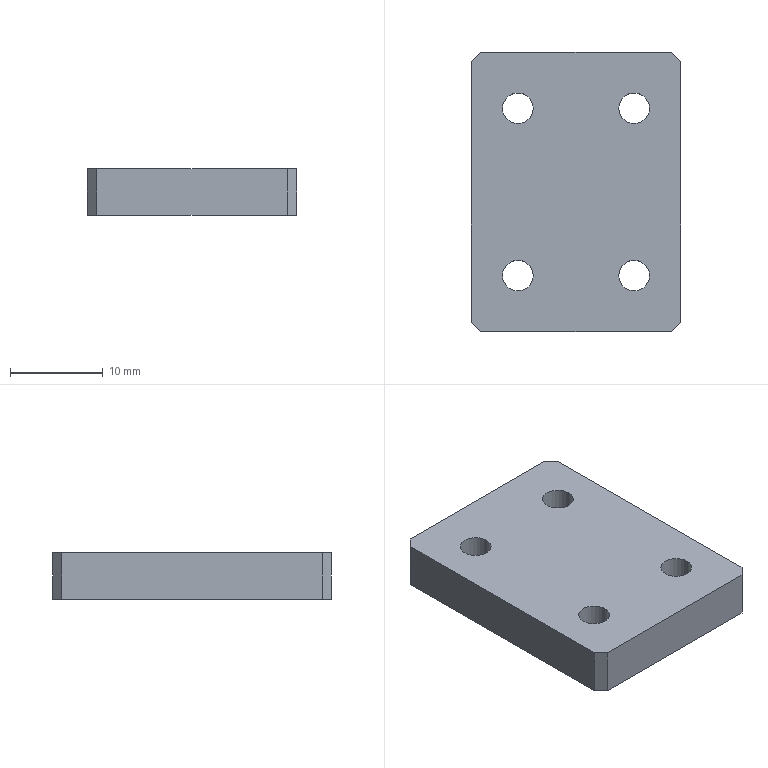Part | STEP file | 01-07 loading cylinder pad plate | 1 solid | 18 faces | box 22.5 x 30 x 5 mm | volume 3194 mm3 | plane 10 | cylinder 8 | commonest cylinder face diameters 3.3 x8
STEP:
#1=CARTESIAN_POINT('',(4.6,-9.,5.));
#2=VERTEX_POINT('',#1);
#3=CARTESIAN_POINT('',(7.9,-9.,5.));
#4=VERTEX_POINT('',#3);
#5=CARTESIAN_POINT('',(6.25,-9.,5.));
#6=DIRECTION('',(0.,0.,1.));
#7=DIRECTION('',(1.,0.,0.));
#8=AXIS2_PLACEMENT_3D('',#5,#6,#7);
#9=CIRCLE('',#8,1.65);
#10=EDGE_CURVE('',#2,#4,#9,.T.);
#11=ORIENTED_EDGE('',*,*,#10,.T.);
#12=CARTESIAN_POINT('',(7.9,-9.,0.));
#13=VERTEX_POINT('',#12);
#14=CARTESIAN_POINT('',(7.9,-9.,0.));
#15=DIRECTION('',(0.,0.,-1.));
#16=VECTOR('',#15,1000.);
#17=LINE('',#14,#16);
#18=EDGE_CURVE('',#4,#13,#17,.T.);
#19=ORIENTED_EDGE('',*,*,#18,.T.);
#20=CARTESIAN_POINT('',(4.6,-9.,0.));
#21=VERTEX_POINT('',#20);
#22=CARTESIAN_POINT('',(6.25,-9.,0.));
#23=DIRECTION('',(0.,0.,-1.));
#24=DIRECTION('',(-1.,0.,0.));
#25=AXIS2_PLACEMENT_3D('',#22,#23,#24);
#26=CIRCLE('',#25,1.65);
#27=EDGE_CURVE('',#13,#21,#26,.T.);
#28=ORIENTED_EDGE('',*,*,#27,.T.);
#29=CARTESIAN_POINT('',(4.6,-9.,0.));
#30=DIRECTION('',(0.,0.,-1.));
#31=VECTOR('',#30,1000.);
#32=LINE('',#29,#31);
#33=EDGE_CURVE('',#2,#21,#32,.T.);
#34=ORIENTED_EDGE('',*,*,#33,.F.);
#35=EDGE_LOOP('',(#11,#19,#28,#34));
#36=FACE_OUTER_BOUND('',#35,.T.);
#37=CARTESIAN_POINT('',(6.25,-9.,0.));
#38=DIRECTION('',(0.,0.,-1.));
#39=DIRECTION('',(-1.,0.,0.));
#40=AXIS2_PLACEMENT_3D('',#37,#38,#39);
#41=CYLINDRICAL_SURFACE('',#40,1.65);
#42=ADVANCED_FACE('',(#36),#41,.F.);
#43=CARTESIAN_POINT('',(-7.9,-9.,5.));
#44=VERTEX_POINT('',#43);
#45=CARTESIAN_POINT('',(-4.6,-9.,5.));
#46=VERTEX_POINT('',#45);
#47=CARTESIAN_POINT('',(-6.25,-9.,5.));
#48=DIRECTION('',(0.,0.,1.));
#49=DIRECTION('',(1.,0.,0.));
#50=AXIS2_PLACEMENT_3D('',#47,#48,#49);
#51=CIRCLE('',#50,1.65);
#52=EDGE_CURVE('',#44,#46,#51,.T.);
#53=ORIENTED_EDGE('',*,*,#52,.T.);
#54=CARTESIAN_POINT('',(-4.6,-9.,0.));
#55=VERTEX_POINT('',#54);
#56=CARTESIAN_POINT('',(-4.6,-9.,0.));
#57=DIRECTION('',(0.,0.,-1.));
#58=VECTOR('',#57,1000.);
#59=LINE('',#56,#58);
#60=EDGE_CURVE('',#46,#55,#59,.T.);
#61=ORIENTED_EDGE('',*,*,#60,.T.);
#62=CARTESIAN_POINT('',(-7.9,-9.,0.));
#63=VERTEX_POINT('',#62);
#64=CARTESIAN_POINT('',(-6.25,-9.,0.));
#65=DIRECTION('',(0.,0.,-1.));
#66=DIRECTION('',(-1.,0.,0.));
#67=AXIS2_PLACEMENT_3D('',#64,#65,#66);
#68=CIRCLE('',#67,1.65);
#69=EDGE_CURVE('',#55,#63,#68,.T.);
#70=ORIENTED_EDGE('',*,*,#69,.T.);
#71=CARTESIAN_POINT('',(-7.9,-9.,0.));
#72=DIRECTION('',(0.,0.,-1.));
#73=VECTOR('',#72,1000.);
#74=LINE('',#71,#73);
#75=EDGE_CURVE('',#44,#63,#74,.T.);
#76=ORIENTED_EDGE('',*,*,#75,.F.);
#77=EDGE_LOOP('',(#53,#61,#70,#76));
#78=FACE_OUTER_BOUND('',#77,.T.);
#79=CARTESIAN_POINT('',(-6.25,-9.,0.));
#80=DIRECTION('',(0.,0.,-1.));
#81=DIRECTION('',(-1.,0.,0.));
#82=AXIS2_PLACEMENT_3D('',#79,#80,#81);
#83=CYLINDRICAL_SURFACE('',#82,1.65);
#84=ADVANCED_FACE('',(#78),#83,.F.);
#85=CARTESIAN_POINT('',(-7.9,9.,5.));
#86=VERTEX_POINT('',#85);
#87=CARTESIAN_POINT('',(-4.6,9.,5.));
#88=VERTEX_POINT('',#87);
#89=CARTESIAN_POINT('',(-6.25,9.,5.));
#90=DIRECTION('',(0.,0.,1.));
#91=DIRECTION('',(1.,0.,0.));
#92=AXIS2_PLACEMENT_3D('',#89,#90,#91);
#93=CIRCLE('',#92,1.65);
#94=EDGE_CURVE('',#86,#88,#93,.T.);
#95=ORIENTED_EDGE('',*,*,#94,.T.);
#96=CARTESIAN_POINT('',(-4.6,9.,0.));
#97=VERTEX_POINT('',#96);
#98=CARTESIAN_POINT('',(-4.6,9.,0.));
#99=DIRECTION('',(0.,0.,-1.));
#100=VECTOR('',#99,1000.);
#101=LINE('',#98,#100);
#102=EDGE_CURVE('',#88,#97,#101,.T.);
#103=ORIENTED_EDGE('',*,*,#102,.T.);
#104=CARTESIAN_POINT('',(-7.9,9.,0.));
#105=VERTEX_POINT('',#104);
#106=CARTESIAN_POINT('',(-6.25,9.,0.));
#107=DIRECTION('',(0.,0.,-1.));
#108=DIRECTION('',(-1.,0.,0.));
#109=AXIS2_PLACEMENT_3D('',#106,#107,#108);
#110=CIRCLE('',#109,1.65);
#111=EDGE_CURVE('',#97,#105,#110,.T.);
#112=ORIENTED_EDGE('',*,*,#111,.T.);
#113=CARTESIAN_POINT('',(-7.9,9.,0.));
#114=DIRECTION('',(0.,0.,-1.));
#115=VECTOR('',#114,1000.);
#116=LINE('',#113,#115);
#117=EDGE_CURVE('',#86,#105,#116,.T.);
#118=ORIENTED_EDGE('',*,*,#117,.F.);
#119=EDGE_LOOP('',(#95,#103,#112,#118));
#120=FACE_OUTER_BOUND('',#119,.T.);
#121=CARTESIAN_POINT('',(-6.25,9.,0.));
#122=DIRECTION('',(0.,0.,-1.));
#123=DIRECTION('',(-1.,0.,0.));
#124=AXIS2_PLACEMENT_3D('',#121,#122,#123);
#125=CYLINDRICAL_SURFACE('',#124,1.65);
#126=ADVANCED_FACE('',(#120),#125,.F.);
#127=CARTESIAN_POINT('',(4.6,9.,5.));
#128=VERTEX_POINT('',#127);
#129=CARTESIAN_POINT('',(7.9,9.,5.));
#130=VERTEX_POINT('',#129);
#131=CARTESIAN_POINT('',(6.25,9.,5.));
#132=DIRECTION('',(0.,0.,1.));
#133=DIRECTION('',(1.,0.,0.));
#134=AXIS2_PLACEMENT_3D('',#131,#132,#133);
#135=CIRCLE('',#134,1.65);
#136=EDGE_CURVE('',#128,#130,#135,.T.);
#137=ORIENTED_EDGE('',*,*,#136,.T.);
#138=CARTESIAN_POINT('',(7.9,9.,0.));
#139=VERTEX_POINT('',#138);
#140=CARTESIAN_POINT('',(7.9,9.,0.));
#141=DIRECTION('',(0.,0.,-1.));
#142=VECTOR('',#141,1000.);
#143=LINE('',#140,#142);
#144=EDGE_CURVE('',#130,#139,#143,.T.);
#145=ORIENTED_EDGE('',*,*,#144,.T.);
#146=CARTESIAN_POINT('',(4.6,9.,0.));
#147=VERTEX_POINT('',#146);
#148=CARTESIAN_POINT('',(6.25,9.,0.));
#149=DIRECTION('',(0.,0.,-1.));
#150=DIRECTION('',(-1.,0.,0.));
#151=AXIS2_PLACEMENT_3D('',#148,#149,#150);
#152=CIRCLE('',#151,1.65);
#153=EDGE_CURVE('',#139,#147,#152,.T.);
#154=ORIENTED_EDGE('',*,*,#153,.T.);
#155=CARTESIAN_POINT('',(4.6,9.,0.));
#156=DIRECTION('',(0.,0.,-1.));
#157=VECTOR('',#156,1000.);
#158=LINE('',#155,#157);
#159=EDGE_CURVE('',#128,#147,#158,.T.);
#160=ORIENTED_EDGE('',*,*,#159,.F.);
#161=EDGE_LOOP('',(#137,#145,#154,#160));
#162=FACE_OUTER_BOUND('',#161,.T.);
#163=CARTESIAN_POINT('',(6.25,9.,0.));
#164=DIRECTION('',(0.,0.,-1.));
#165=DIRECTION('',(-1.,0.,0.));
#166=AXIS2_PLACEMENT_3D('',#163,#164,#165);
#167=CYLINDRICAL_SURFACE('',#166,1.65);
#168=ADVANCED_FACE('',(#162),#167,.F.);
#169=CARTESIAN_POINT('',(11.25,-14.,5.));
#170=VERTEX_POINT('',#169);
#171=CARTESIAN_POINT('',(11.25,14.,5.));
#172=VERTEX_POINT('',#171);
#173=CARTESIAN_POINT('',(11.25,15.,5.));
#174=DIRECTION('',(0.,1.,0.));
#175=VECTOR('',#174,1000.);
#176=LINE('',#173,#175);
#177=EDGE_CURVE('',#170,#172,#176,.T.);
#178=ORIENTED_EDGE('',*,*,#177,.F.);
#179=CARTESIAN_POINT('',(11.25,-14.,0.));
#180=VERTEX_POINT('',#179);
#181=CARTESIAN_POINT('',(11.25,-14.,5.));
#182=DIRECTION('',(0.,0.,-1.));
#183=VECTOR('',#182,1000.);
#184=LINE('',#181,#183);
#185=EDGE_CURVE('',#170,#180,#184,.T.);
#186=ORIENTED_EDGE('',*,*,#185,.T.);
#187=CARTESIAN_POINT('',(11.25,14.,0.));
#188=VERTEX_POINT('',#187);
#189=CARTESIAN_POINT('',(11.25,15.,0.));
#190=DIRECTION('',(0.,1.,0.));
#191=VECTOR('',#190,1000.);
#192=LINE('',#189,#191);
#193=EDGE_CURVE('',#180,#188,#192,.T.);
#194=ORIENTED_EDGE('',*,*,#193,.T.);
#195=CARTESIAN_POINT('',(11.25,14.,5.));
#196=DIRECTION('',(0.,0.,1.));
#197=VECTOR('',#196,1000.);
#198=LINE('',#195,#197);
#199=EDGE_CURVE('',#188,#172,#198,.T.);
#200=ORIENTED_EDGE('',*,*,#199,.T.);
#201=EDGE_LOOP('',(#178,#186,#194,#200));
#202=FACE_OUTER_BOUND('',#201,.T.);
#203=CARTESIAN_POINT('',(11.25,15.,5.));
#204=DIRECTION('',(-1.,0.,0.));
#205=DIRECTION('',(0.,-1.,0.));
#206=AXIS2_PLACEMENT_3D('',#203,#204,#205);
#207=PLANE('',#206);
#208=ADVANCED_FACE('',(#202),#207,.F.);
#209=CARTESIAN_POINT('',(10.25,15.,0.));
#210=VERTEX_POINT('',#209);
#211=CARTESIAN_POINT('',(-10.25,15.,0.));
#212=VERTEX_POINT('',#211);
#213=CARTESIAN_POINT('',(-11.25,15.,0.));
#214=DIRECTION('',(-1.,0.,0.));
#215=VECTOR('',#214,1000.);
#216=LINE('',#213,#215);
#217=EDGE_CURVE('',#210,#212,#216,.T.);
#218=ORIENTED_EDGE('',*,*,#217,.T.);
#219=CARTESIAN_POINT('',(-10.25,15.,5.));
#220=VERTEX_POINT('',#219);
#221=CARTESIAN_POINT('',(-10.25,15.,5.));
#222=DIRECTION('',(0.,0.,1.));
#223=VECTOR('',#222,1000.);
#224=LINE('',#221,#223);
#225=EDGE_CURVE('',#212,#220,#224,.T.);
#226=ORIENTED_EDGE('',*,*,#225,.T.);
#227=CARTESIAN_POINT('',(10.25,15.,5.));
#228=VERTEX_POINT('',#227);
#229=CARTESIAN_POINT('',(-11.25,15.,5.));
#230=DIRECTION('',(-1.,0.,0.));
#231=VECTOR('',#230,1000.);
#232=LINE('',#229,#231);
#233=EDGE_CURVE('',#228,#220,#232,.T.);
#234=ORIENTED_EDGE('',*,*,#233,.F.);
#235=CARTESIAN_POINT('',(10.25,15.,5.));
#236=DIRECTION('',(0.,0.,-1.));
#237=VECTOR('',#236,1000.);
#238=LINE('',#235,#237);
#239=EDGE_CURVE('',#228,#210,#238,.T.);
#240=ORIENTED_EDGE('',*,*,#239,.T.);
#241=EDGE_LOOP('',(#218,#226,#234,#240));
#242=FACE_OUTER_BOUND('',#241,.T.);
#243=CARTESIAN_POINT('',(-11.25,15.,5.));
#244=DIRECTION('',(0.,-1.,0.));
#245=DIRECTION('',(0.,0.,-1.));
#246=AXIS2_PLACEMENT_3D('',#243,#244,#245);
#247=PLANE('',#246);
#248=ADVANCED_FACE('',(#242),#247,.F.);
#249=CARTESIAN_POINT('',(-11.25,14.,5.));
#250=VERTEX_POINT('',#249);
#251=CARTESIAN_POINT('',(-11.25,-14.,5.));
#252=VERTEX_POINT('',#251);
#253=CARTESIAN_POINT('',(-11.25,15.,5.));
#254=DIRECTION('',(0.,-1.,0.));
#255=VECTOR('',#254,1000.);
#256=LINE('',#253,#255);
#257=EDGE_CURVE('',#250,#252,#256,.T.);
#258=ORIENTED_EDGE('',*,*,#257,.F.);
#259=CARTESIAN_POINT('',(-11.25,14.,0.));
#260=VERTEX_POINT('',#259);
#261=CARTESIAN_POINT('',(-11.25,14.,5.));
#262=DIRECTION('',(0.,0.,-1.));
#263=VECTOR('',#262,1000.);
#264=LINE('',#261,#263);
#265=EDGE_CURVE('',#250,#260,#264,.T.);
#266=ORIENTED_EDGE('',*,*,#265,.T.);
#267=CARTESIAN_POINT('',(-11.25,-14.,0.));
#268=VERTEX_POINT('',#267);
#269=CARTESIAN_POINT('',(-11.25,15.,0.));
#270=DIRECTION('',(0.,-1.,0.));
#271=VECTOR('',#270,1000.);
#272=LINE('',#269,#271);
#273=EDGE_CURVE('',#260,#268,#272,.T.);
#274=ORIENTED_EDGE('',*,*,#273,.T.);
#275=CARTESIAN_POINT('',(-11.25,-14.,5.));
#276=DIRECTION('',(0.,0.,1.));
#277=VECTOR('',#276,1000.);
#278=LINE('',#275,#277);
#279=EDGE_CURVE('',#268,#252,#278,.T.);
#280=ORIENTED_EDGE('',*,*,#279,.T.);
#281=EDGE_LOOP('',(#258,#266,#274,#280));
#282=FACE_OUTER_BOUND('',#281,.T.);
#283=CARTESIAN_POINT('',(-11.25,15.,5.));
#284=DIRECTION('',(1.,0.,0.));
#285=DIRECTION('',(0.,1.,0.));
#286=AXIS2_PLACEMENT_3D('',#283,#284,#285);
#287=PLANE('',#286);
#288=ADVANCED_FACE('',(#282),#287,.F.);
#289=CARTESIAN_POINT('',(-10.25,-15.,5.));
#290=VERTEX_POINT('',#289);
#291=CARTESIAN_POINT('',(10.25,-15.,5.));
#292=VERTEX_POINT('',#291);
#293=CARTESIAN_POINT('',(-11.25,-15.,5.));
#294=DIRECTION('',(1.,0.,0.));
#295=VECTOR('',#294,1000.);
#296=LINE('',#293,#295);
#297=EDGE_CURVE('',#290,#292,#296,.T.);
#298=ORIENTED_EDGE('',*,*,#297,.F.);
#299=CARTESIAN_POINT('',(-10.25,-15.,0.));
#300=VERTEX_POINT('',#299);
#301=CARTESIAN_POINT('',(-10.25,-15.,5.));
#302=DIRECTION('',(0.,0.,-1.));
#303=VECTOR('',#302,1000.);
#304=LINE('',#301,#303);
#305=EDGE_CURVE('',#290,#300,#304,.T.);
#306=ORIENTED_EDGE('',*,*,#305,.T.);
#307=CARTESIAN_POINT('',(10.25,-15.,0.));
#308=VERTEX_POINT('',#307);
#309=CARTESIAN_POINT('',(-11.25,-15.,0.));
#310=DIRECTION('',(1.,0.,0.));
#311=VECTOR('',#310,1000.);
#312=LINE('',#309,#311);
#313=EDGE_CURVE('',#300,#308,#312,.T.);
#314=ORIENTED_EDGE('',*,*,#313,.T.);
#315=CARTESIAN_POINT('',(10.25,-15.,5.));
#316=DIRECTION('',(0.,0.,1.));
#317=VECTOR('',#316,1000.);
#318=LINE('',#315,#317);
#319=EDGE_CURVE('',#308,#292,#318,.T.);
#320=ORIENTED_EDGE('',*,*,#319,.T.);
#321=EDGE_LOOP('',(#298,#306,#314,#320));
#322=FACE_OUTER_BOUND('',#321,.T.);
#323=CARTESIAN_POINT('',(-11.25,-15.,5.));
#324=DIRECTION('',(0.,1.,0.));
#325=DIRECTION('',(0.,0.,1.));
#326=AXIS2_PLACEMENT_3D('',#323,#324,#325);
#327=PLANE('',#326);
#328=ADVANCED_FACE('',(#322),#327,.F.);
#329=ORIENTED_EDGE('',*,*,#10,.F.);
#330=CARTESIAN_POINT('',(6.25,-9.,5.));
#331=DIRECTION('',(0.,0.,1.));
#332=DIRECTION('',(1.,0.,0.));
#333=AXIS2_PLACEMENT_3D('',#330,#331,#332);
#334=CIRCLE('',#333,1.65);
#335=EDGE_CURVE('',#4,#2,#334,.T.);
#336=ORIENTED_EDGE('',*,*,#335,.F.);
#337=EDGE_LOOP('',(#329,#336));
#338=FACE_BOUND('',#337,.T.);
#339=ORIENTED_EDGE('',*,*,#52,.F.);
#340=CARTESIAN_POINT('',(-6.25,-9.,5.));
#341=DIRECTION('',(0.,0.,1.));
#342=DIRECTION('',(1.,0.,0.));
#343=AXIS2_PLACEMENT_3D('',#340,#341,#342);
#344=CIRCLE('',#343,1.65);
#345=EDGE_CURVE('',#46,#44,#344,.T.);
#346=ORIENTED_EDGE('',*,*,#345,.F.);
#347=EDGE_LOOP('',(#339,#346));
#348=FACE_BOUND('',#347,.T.);
#349=ORIENTED_EDGE('',*,*,#94,.F.);
#350=CARTESIAN_POINT('',(-6.25,9.,5.));
#351=DIRECTION('',(0.,0.,1.));
#352=DIRECTION('',(1.,0.,0.));
#353=AXIS2_PLACEMENT_3D('',#350,#351,#352);
#354=CIRCLE('',#353,1.65);
#355=EDGE_CURVE('',#88,#86,#354,.T.);
#356=ORIENTED_EDGE('',*,*,#355,.F.);
#357=EDGE_LOOP('',(#349,#356));
#358=FACE_BOUND('',#357,.T.);
#359=ORIENTED_EDGE('',*,*,#136,.F.);
#360=CARTESIAN_POINT('',(6.25,9.,5.));
#361=DIRECTION('',(0.,0.,1.));
#362=DIRECTION('',(1.,0.,0.));
#363=AXIS2_PLACEMENT_3D('',#360,#361,#362);
#364=CIRCLE('',#363,1.65);
#365=EDGE_CURVE('',#130,#128,#364,.T.);
#366=ORIENTED_EDGE('',*,*,#365,.F.);
#367=EDGE_LOOP('',(#359,#366));
#368=FACE_BOUND('',#367,.T.);
#369=ORIENTED_EDGE('',*,*,#233,.T.);
#370=CARTESIAN_POINT('',(-14.5,10.75,5.));
#371=DIRECTION('',(-0.7071,-0.7071,0.));
#372=VECTOR('',#371,1000.);
#373=LINE('',#370,#372);
#374=EDGE_CURVE('',#220,#250,#373,.T.);
#375=ORIENTED_EDGE('',*,*,#374,.T.);
#376=ORIENTED_EDGE('',*,*,#257,.T.);
#377=CARTESIAN_POINT('',(0.5,-25.75,5.));
#378=DIRECTION('',(0.7071,-0.7071,0.));
#379=VECTOR('',#378,1000.);
#380=LINE('',#377,#379);
#381=EDGE_CURVE('',#252,#290,#380,.T.);
#382=ORIENTED_EDGE('',*,*,#381,.T.);
#383=ORIENTED_EDGE('',*,*,#297,.T.);
#384=CARTESIAN_POINT('',(10.75,-14.5,5.));
#385=DIRECTION('',(0.7071,0.7071,0.));
#386=VECTOR('',#385,1000.);
#387=LINE('',#384,#386);
#388=EDGE_CURVE('',#292,#170,#387,.T.);
#389=ORIENTED_EDGE('',*,*,#388,.T.);
#390=ORIENTED_EDGE('',*,*,#177,.T.);
#391=CARTESIAN_POINT('',(25.75,-0.5,5.));
#392=DIRECTION('',(-0.7071,0.7071,0.));
#393=VECTOR('',#392,1000.);
#394=LINE('',#391,#393);
#395=EDGE_CURVE('',#172,#228,#394,.T.);
#396=ORIENTED_EDGE('',*,*,#395,.T.);
#397=EDGE_LOOP('',(#369,#375,#376,#382,#383,#389,#390,#396));
#398=FACE_OUTER_BOUND('',#397,.T.);
#399=CARTESIAN_POINT('',(11.25,-15.,5.));
#400=DIRECTION('',(0.,0.,1.));
#401=DIRECTION('',(1.,0.,0.));
#402=AXIS2_PLACEMENT_3D('',#399,#400,#401);
#403=PLANE('',#402);
#404=ADVANCED_FACE('',(#338,#348,#358,#368,#398),#403,.T.);
#405=CARTESIAN_POINT('',(6.25,-9.,0.));
#406=DIRECTION('',(0.,0.,-1.));
#407=DIRECTION('',(-1.,0.,0.));
#408=AXIS2_PLACEMENT_3D('',#405,#406,#407);
#409=CIRCLE('',#408,1.65);
#410=EDGE_CURVE('',#21,#13,#409,.T.);
#411=ORIENTED_EDGE('',*,*,#410,.F.);
#412=ORIENTED_EDGE('',*,*,#27,.F.);
#413=EDGE_LOOP('',(#411,#412));
#414=FACE_BOUND('',#413,.T.);
#415=CARTESIAN_POINT('',(-6.25,-9.,0.));
#416=DIRECTION('',(0.,0.,-1.));
#417=DIRECTION('',(-1.,0.,0.));
#418=AXIS2_PLACEMENT_3D('',#415,#416,#417);
#419=CIRCLE('',#418,1.65);
#420=EDGE_CURVE('',#63,#55,#419,.T.);
#421=ORIENTED_EDGE('',*,*,#420,.F.);
#422=ORIENTED_EDGE('',*,*,#69,.F.);
#423=EDGE_LOOP('',(#421,#422));
#424=FACE_BOUND('',#423,.T.);
#425=CARTESIAN_POINT('',(-6.25,9.,0.));
#426=DIRECTION('',(0.,0.,-1.));
#427=DIRECTION('',(-1.,0.,0.));
#428=AXIS2_PLACEMENT_3D('',#425,#426,#427);
#429=CIRCLE('',#428,1.65);
#430=EDGE_CURVE('',#105,#97,#429,.T.);
#431=ORIENTED_EDGE('',*,*,#430,.F.);
#432=ORIENTED_EDGE('',*,*,#111,.F.);
#433=EDGE_LOOP('',(#431,#432));
#434=FACE_BOUND('',#433,.T.);
#435=CARTESIAN_POINT('',(6.25,9.,0.));
#436=DIRECTION('',(0.,0.,-1.));
#437=DIRECTION('',(-1.,0.,0.));
#438=AXIS2_PLACEMENT_3D('',#435,#436,#437);
#439=CIRCLE('',#438,1.65);
#440=EDGE_CURVE('',#147,#139,#439,.T.);
#441=ORIENTED_EDGE('',*,*,#440,.F.);
#442=ORIENTED_EDGE('',*,*,#153,.F.);
#443=EDGE_LOOP('',(#441,#442));
#444=FACE_BOUND('',#443,.T.);
#445=ORIENTED_EDGE('',*,*,#273,.F.);
#446=CARTESIAN_POINT('',(-11.25,14.,0.));
#447=DIRECTION('',(0.7071,0.7071,0.));
#448=VECTOR('',#447,1000.);
#449=LINE('',#446,#448);
#450=EDGE_CURVE('',#260,#212,#449,.T.);
#451=ORIENTED_EDGE('',*,*,#450,.T.);
#452=ORIENTED_EDGE('',*,*,#217,.F.);
#453=CARTESIAN_POINT('',(10.25,15.,0.));
#454=DIRECTION('',(0.7071,-0.7071,0.));
#455=VECTOR('',#454,1000.);
#456=LINE('',#453,#455);
#457=EDGE_CURVE('',#210,#188,#456,.T.);
#458=ORIENTED_EDGE('',*,*,#457,.T.);
#459=ORIENTED_EDGE('',*,*,#193,.F.);
#460=CARTESIAN_POINT('',(11.25,-14.,0.));
#461=DIRECTION('',(-0.7071,-0.7071,0.));
#462=VECTOR('',#461,1000.);
#463=LINE('',#460,#462);
#464=EDGE_CURVE('',#180,#308,#463,.T.);
#465=ORIENTED_EDGE('',*,*,#464,.T.);
#466=ORIENTED_EDGE('',*,*,#313,.F.);
#467=CARTESIAN_POINT('',(-10.25,-15.,0.));
#468=DIRECTION('',(-0.7071,0.7071,0.));
#469=VECTOR('',#468,1000.);
#470=LINE('',#467,#469);
#471=EDGE_CURVE('',#300,#268,#470,.T.);
#472=ORIENTED_EDGE('',*,*,#471,.T.);
#473=EDGE_LOOP('',(#445,#451,#452,#458,#459,#465,#466,#472));
#474=FACE_OUTER_BOUND('',#473,.T.);
#475=CARTESIAN_POINT('',(11.25,-15.,0.));
#476=DIRECTION('',(0.,0.,1.));
#477=DIRECTION('',(1.,0.,0.));
#478=AXIS2_PLACEMENT_3D('',#475,#476,#477);
#479=PLANE('',#478);
#480=ADVANCED_FACE('',(#414,#424,#434,#444,#474),#479,.F.);
#481=ORIENTED_EDGE('',*,*,#144,.F.);
#482=ORIENTED_EDGE('',*,*,#365,.T.);
#483=ORIENTED_EDGE('',*,*,#159,.T.);
#484=ORIENTED_EDGE('',*,*,#440,.T.);
#485=EDGE_LOOP('',(#481,#482,#483,#484));
#486=FACE_OUTER_BOUND('',#485,.T.);
#487=CARTESIAN_POINT('',(6.25,9.,0.));
#488=DIRECTION('',(0.,0.,-1.));
#489=DIRECTION('',(-1.,0.,0.));
#490=AXIS2_PLACEMENT_3D('',#487,#488,#489);
#491=CYLINDRICAL_SURFACE('',#490,1.65);
#492=ADVANCED_FACE('',(#486),#491,.F.);
#493=ORIENTED_EDGE('',*,*,#102,.F.);
#494=ORIENTED_EDGE('',*,*,#355,.T.);
#495=ORIENTED_EDGE('',*,*,#117,.T.);
#496=ORIENTED_EDGE('',*,*,#430,.T.);
#497=EDGE_LOOP('',(#493,#494,#495,#496));
#498=FACE_OUTER_BOUND('',#497,.T.);
#499=CARTESIAN_POINT('',(-6.25,9.,0.));
#500=DIRECTION('',(0.,0.,-1.));
#501=DIRECTION('',(-1.,0.,0.));
#502=AXIS2_PLACEMENT_3D('',#499,#500,#501);
#503=CYLINDRICAL_SURFACE('',#502,1.65);
#504=ADVANCED_FACE('',(#498),#503,.F.);
#505=ORIENTED_EDGE('',*,*,#60,.F.);
#506=ORIENTED_EDGE('',*,*,#345,.T.);
#507=ORIENTED_EDGE('',*,*,#75,.T.);
#508=ORIENTED_EDGE('',*,*,#420,.T.);
#509=EDGE_LOOP('',(#505,#506,#507,#508));
#510=FACE_OUTER_BOUND('',#509,.T.);
#511=CARTESIAN_POINT('',(-6.25,-9.,0.));
#512=DIRECTION('',(0.,0.,-1.));
#513=DIRECTION('',(-1.,0.,0.));
#514=AXIS2_PLACEMENT_3D('',#511,#512,#513);
#515=CYLINDRICAL_SURFACE('',#514,1.65);
#516=ADVANCED_FACE('',(#510),#515,.F.);
#517=ORIENTED_EDGE('',*,*,#18,.F.);
#518=ORIENTED_EDGE('',*,*,#335,.T.);
#519=ORIENTED_EDGE('',*,*,#33,.T.);
#520=ORIENTED_EDGE('',*,*,#410,.T.);
#521=EDGE_LOOP('',(#517,#518,#519,#520));
#522=FACE_OUTER_BOUND('',#521,.T.);
#523=CARTESIAN_POINT('',(6.25,-9.,0.));
#524=DIRECTION('',(0.,0.,-1.));
#525=DIRECTION('',(-1.,0.,0.));
#526=AXIS2_PLACEMENT_3D('',#523,#524,#525);
#527=CYLINDRICAL_SURFACE('',#526,1.65);
#528=ADVANCED_FACE('',(#522),#527,.F.);
#529=ORIENTED_EDGE('',*,*,#374,.F.);
#530=ORIENTED_EDGE('',*,*,#225,.F.);
#531=ORIENTED_EDGE('',*,*,#450,.F.);
#532=ORIENTED_EDGE('',*,*,#265,.F.);
#533=EDGE_LOOP('',(#529,#530,#531,#532));
#534=FACE_OUTER_BOUND('',#533,.T.);
#535=CARTESIAN_POINT('',(-11.25,14.,5.));
#536=DIRECTION('',(0.7071,-0.7071,0.));
#537=DIRECTION('',(0.7071,0.7071,0.));
#538=AXIS2_PLACEMENT_3D('',#535,#536,#537);
#539=PLANE('',#538);
#540=ADVANCED_FACE('',(#534),#539,.F.);
#541=ORIENTED_EDGE('',*,*,#381,.F.);
#542=ORIENTED_EDGE('',*,*,#279,.F.);
#543=ORIENTED_EDGE('',*,*,#471,.F.);
#544=ORIENTED_EDGE('',*,*,#305,.F.);
#545=EDGE_LOOP('',(#541,#542,#543,#544));
#546=FACE_OUTER_BOUND('',#545,.T.);
#547=CARTESIAN_POINT('',(-10.25,-15.,5.));
#548=DIRECTION('',(0.7071,0.7071,0.));
#549=DIRECTION('',(-0.7071,0.7071,0.));
#550=AXIS2_PLACEMENT_3D('',#547,#548,#549);
#551=PLANE('',#550);
#552=ADVANCED_FACE('',(#546),#551,.F.);
#553=ORIENTED_EDGE('',*,*,#388,.F.);
#554=ORIENTED_EDGE('',*,*,#319,.F.);
#555=ORIENTED_EDGE('',*,*,#464,.F.);
#556=ORIENTED_EDGE('',*,*,#185,.F.);
#557=EDGE_LOOP('',(#553,#554,#555,#556));
#558=FACE_OUTER_BOUND('',#557,.T.);
#559=CARTESIAN_POINT('',(11.25,-14.,5.));
#560=DIRECTION('',(-0.7071,0.7071,0.));
#561=DIRECTION('',(-0.7071,-0.7071,0.));
#562=AXIS2_PLACEMENT_3D('',#559,#560,#561);
#563=PLANE('',#562);
#564=ADVANCED_FACE('',(#558),#563,.F.);
#565=ORIENTED_EDGE('',*,*,#395,.F.);
#566=ORIENTED_EDGE('',*,*,#199,.F.);
#567=ORIENTED_EDGE('',*,*,#457,.F.);
#568=ORIENTED_EDGE('',*,*,#239,.F.);
#569=EDGE_LOOP('',(#565,#566,#567,#568));
#570=FACE_OUTER_BOUND('',#569,.T.);
#571=CARTESIAN_POINT('',(10.25,15.,5.));
#572=DIRECTION('',(-0.7071,-0.7071,0.));
#573=DIRECTION('',(0.7071,-0.7071,0.));
#574=AXIS2_PLACEMENT_3D('',#571,#572,#573);
#575=PLANE('',#574);
#576=ADVANCED_FACE('',(#570),#575,.F.);
#577=CLOSED_SHELL('',(#42,#84,#126,#168,#208,#248,#288,#328,#404,#480,#492,#504,#516,#528,#540,#552,#564,#576));
#578=MANIFOLD_SOLID_BREP('',#577);
#579=CARTESIAN_POINT('',(0.,0.,0.));
#580=DIRECTION('',(0.,0.,1.));
#581=DIRECTION('',(1.,0.,0.));
#582=AXIS2_PLACEMENT_3D('',#579,#580,#581);
#583=(LENGTH_UNIT()NAMED_UNIT(*)SI_UNIT(.MILLI.,.METRE.));
#584=UNCERTAINTY_MEASURE_WITH_UNIT(LENGTH_MEASURE(0.00001),#583,'','');
#585=(NAMED_UNIT(*)PLANE_ANGLE_UNIT()SI_UNIT($,.RADIAN.));
#586=(NAMED_UNIT(*)SI_UNIT($,.STERADIAN.)SOLID_ANGLE_UNIT());
#587=(GEOMETRIC_REPRESENTATION_CONTEXT(3)GLOBAL_UNCERTAINTY_ASSIGNED_CONTEXT((#584))GLOBAL_UNIT_ASSIGNED_CONTEXT((#583,#585,#586))REPRESENTATION_CONTEXT('',''));
#588=ADVANCED_BREP_SHAPE_REPRESENTATION('',(#578,#582),#587);